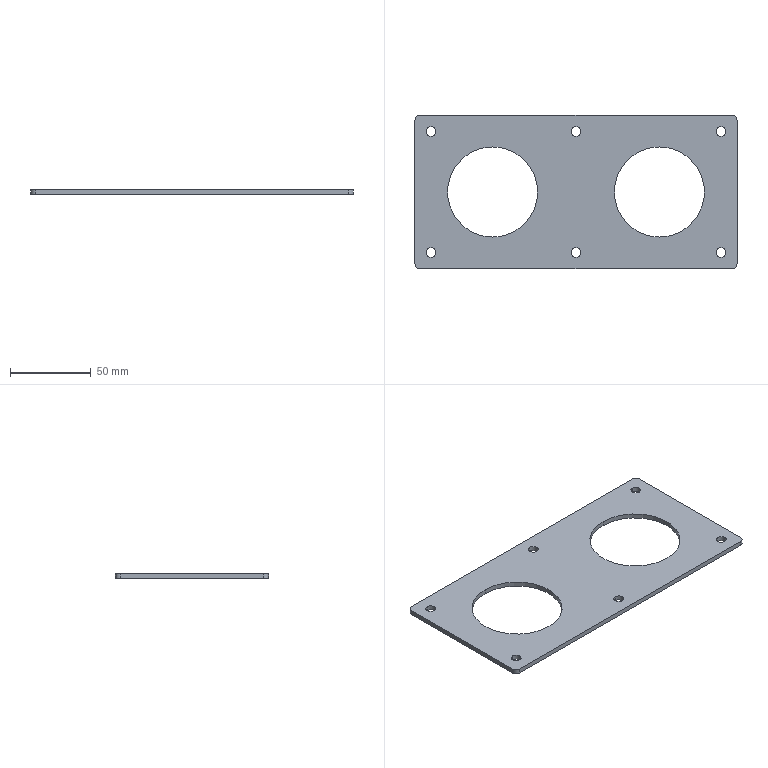Part | STEP file | HESS-408-70-15W-D-8-electrical box lower closing plate | 1 solid | 26 faces | box 200 x 95 x 3 mm | volume 41690 mm3 | cylinder 20 | plane 6 | commonest cylinder face diameters 6 x16 56 x4